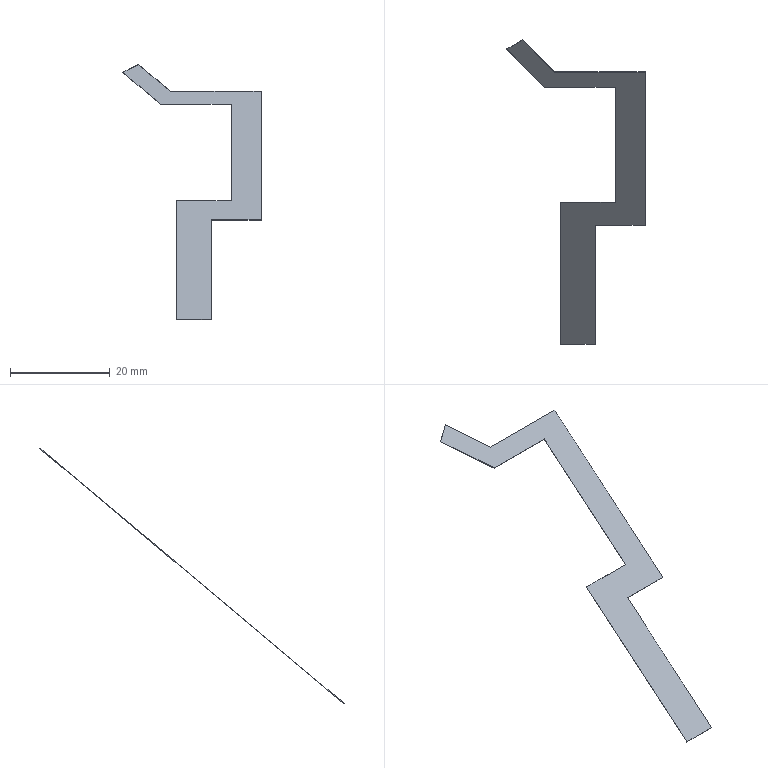Part | SolidWorks | features BaseBody 1 | 1 solid | 15 faces | box 27.714 x 60.861 x 51.086 mm | volume 46.633 mm3 | plane 15
STEP:
#1=CARTESIAN_POINT('',(-706.97,699.765,404.599));
#2=VERTEX_POINT('',#1);
#3=CARTESIAN_POINT('',(-710.165,697.921,403.051));
#4=VERTEX_POINT('',#3);
#5=CARTESIAN_POINT('',(-706.97,699.765,404.599));
#6=DIRECTION('',(-0.7986,-0.461,-0.3868));
#7=VECTOR('',#6,1000.);
#8=LINE('',#5,#7);
#9=EDGE_CURVE('',#2,#4,#8,.T.);
#10=ORIENTED_EDGE('',*,*,#9,.T.);
#11=CARTESIAN_POINT('',(-710.165,697.873,403.109));
#12=VERTEX_POINT('',#11);
#13=CARTESIAN_POINT('',(-710.165,697.873,403.109));
#14=DIRECTION('',(-0.000000993,0.6428,-0.766));
#15=VECTOR('',#14,1000.);
#16=LINE('',#13,#15);
#17=EDGE_CURVE('',#12,#4,#16,.T.);
#18=ORIENTED_EDGE('',*,*,#17,.F.);
#19=CARTESIAN_POINT('',(-706.97,699.717,404.656));
#20=VERTEX_POINT('',#19);
#21=CARTESIAN_POINT('',(-710.165,697.873,403.109));
#22=DIRECTION('',(0.7986,0.461,0.3868));
#23=VECTOR('',#22,1000.);
#24=LINE('',#21,#23);
#25=EDGE_CURVE('',#12,#20,#24,.T.);
#26=ORIENTED_EDGE('',*,*,#25,.T.);
#27=CARTESIAN_POINT('',(-706.97,699.765,404.599));
#28=DIRECTION('',(0.000000993,-0.6428,0.766));
#29=VECTOR('',#28,1000.);
#30=LINE('',#27,#29);
#31=EDGE_CURVE('',#2,#20,#30,.T.);
#32=ORIENTED_EDGE('',*,*,#31,.F.);
#33=EDGE_LOOP('',(#10,#18,#26,#32));
#34=FACE_OUTER_BOUND('',#33,.T.);
#35=CARTESIAN_POINT('',(-710.165,697.921,403.051));
#36=DIRECTION('',(0.6018,-0.6118,-0.5134));
#37=DIRECTION('',(0.7986,0.461,0.3868));
#38=AXIS2_PLACEMENT_3D('',#35,#36,#37);
#39=PLANE('',#38);
#40=ADVANCED_FACE('',(#34),#39,.F.);
#41=CARTESIAN_POINT('',(-700.651,693.342,399.208));
#42=VERTEX_POINT('',#41);
#43=CARTESIAN_POINT('',(-700.651,693.342,399.208));
#44=DIRECTION('',(-0.6018,0.6118,0.5134));
#45=VECTOR('',#44,1000.);
#46=LINE('',#43,#45);
#47=EDGE_CURVE('',#42,#2,#46,.T.);
#48=ORIENTED_EDGE('',*,*,#47,.T.);
#49=ORIENTED_EDGE('',*,*,#31,.T.);
#50=CARTESIAN_POINT('',(-700.651,693.293,399.266));
#51=VERTEX_POINT('',#50);
#52=CARTESIAN_POINT('',(-706.97,699.717,404.656));
#53=DIRECTION('',(0.6018,-0.6118,-0.5134));
#54=VECTOR('',#53,1000.);
#55=LINE('',#52,#54);
#56=EDGE_CURVE('',#20,#51,#55,.T.);
#57=ORIENTED_EDGE('',*,*,#56,.T.);
#58=CARTESIAN_POINT('',(-700.651,693.342,399.208));
#59=DIRECTION('',(0.000000993,-0.6428,0.766));
#60=VECTOR('',#59,1000.);
#61=LINE('',#58,#60);
#62=EDGE_CURVE('',#42,#51,#61,.T.);
#63=ORIENTED_EDGE('',*,*,#62,.F.);
#64=EDGE_LOOP('',(#48,#49,#57,#63));
#65=FACE_OUTER_BOUND('',#64,.T.);
#66=CARTESIAN_POINT('',(-706.97,699.765,404.599));
#67=DIRECTION('',(-0.7986,-0.461,-0.3868));
#68=DIRECTION('',(0.6018,-0.6118,-0.5134));
#69=AXIS2_PLACEMENT_3D('',#66,#67,#68);
#70=PLANE('',#69);
#71=ADVANCED_FACE('',(#65),#70,.F.);
#72=CARTESIAN_POINT('',(-688.451,693.342,399.208));
#73=VERTEX_POINT('',#72);
#74=CARTESIAN_POINT('',(-688.451,693.342,399.208));
#75=DIRECTION('',(-1.,-0.000001868,-0.000000272));
#76=VECTOR('',#75,1000.);
#77=LINE('',#74,#76);
#78=EDGE_CURVE('',#73,#42,#77,.T.);
#79=ORIENTED_EDGE('',*,*,#78,.T.);
#80=ORIENTED_EDGE('',*,*,#62,.T.);
#81=CARTESIAN_POINT('',(-688.451,693.293,399.266));
#82=VERTEX_POINT('',#81);
#83=CARTESIAN_POINT('',(-700.651,693.293,399.266));
#84=DIRECTION('',(1.,0.000001868,0.000000272));
#85=VECTOR('',#84,1000.);
#86=LINE('',#83,#85);
#87=EDGE_CURVE('',#51,#82,#86,.T.);
#88=ORIENTED_EDGE('',*,*,#87,.T.);
#89=CARTESIAN_POINT('',(-688.451,693.293,399.266));
#90=DIRECTION('',(-0.000000993,0.6428,-0.766));
#91=VECTOR('',#90,1000.);
#92=LINE('',#89,#91);
#93=EDGE_CURVE('',#82,#73,#92,.T.);
#94=ORIENTED_EDGE('',*,*,#93,.T.);
#95=EDGE_LOOP('',(#79,#80,#88,#94));
#96=FACE_OUTER_BOUND('',#95,.T.);
#97=CARTESIAN_POINT('',(-700.651,693.342,399.208));
#98=DIRECTION('',(0.000001866,-0.766,-0.6428));
#99=DIRECTION('',(1.,0.000002068,0.000000439));
#100=AXIS2_PLACEMENT_3D('',#97,#98,#99);
#101=PLANE('',#100);
#102=ADVANCED_FACE('',(#96),#101,.F.);
#103=CARTESIAN_POINT('',(-682.451,693.342,399.208));
#104=VERTEX_POINT('',#103);
#105=CARTESIAN_POINT('',(-682.451,693.342,399.208));
#106=DIRECTION('',(-1.,-0.000001661,-0.000000098));
#107=VECTOR('',#106,1000.);
#108=LINE('',#105,#107);
#109=EDGE_CURVE('',#104,#73,#108,.T.);
#110=ORIENTED_EDGE('',*,*,#109,.T.);
#111=ORIENTED_EDGE('',*,*,#93,.F.);
#112=CARTESIAN_POINT('',(-682.451,693.294,399.266));
#113=VERTEX_POINT('',#112);
#114=CARTESIAN_POINT('',(-688.451,693.293,399.266));
#115=DIRECTION('',(1.,0.000001661,0.000000098));
#116=VECTOR('',#115,1000.);
#117=LINE('',#114,#116);
#118=EDGE_CURVE('',#82,#113,#117,.T.);
#119=ORIENTED_EDGE('',*,*,#118,.T.);
#120=CARTESIAN_POINT('',(-682.451,693.294,399.266));
#121=DIRECTION('',(-0.000000993,0.6428,-0.766));
#122=VECTOR('',#121,1000.);
#123=LINE('',#120,#122);
#124=EDGE_CURVE('',#113,#104,#123,.T.);
#125=ORIENTED_EDGE('',*,*,#124,.T.);
#126=EDGE_LOOP('',(#110,#111,#119,#125));
#127=FACE_OUTER_BOUND('',#126,.T.);
#128=CARTESIAN_POINT('',(-688.451,693.342,399.208));
#129=DIRECTION('',(0.000001286,-0.766,-0.6428));
#130=DIRECTION('',(0.000000993,-0.6428,0.766));
#131=AXIS2_PLACEMENT_3D('',#128,#129,#130);
#132=PLANE('',#131);
#133=ADVANCED_FACE('',(#127),#132,.F.);
#134=CARTESIAN_POINT('',(-682.451,662.7,373.497));
#135=VERTEX_POINT('',#134);
#136=CARTESIAN_POINT('',(-682.451,662.7,373.497));
#137=DIRECTION('',(-0.000001286,0.766,0.6428));
#138=VECTOR('',#137,1000.);
#139=LINE('',#136,#138);
#140=EDGE_CURVE('',#135,#104,#139,.T.);
#141=ORIENTED_EDGE('',*,*,#140,.T.);
#142=ORIENTED_EDGE('',*,*,#124,.F.);
#143=CARTESIAN_POINT('',(-682.451,662.652,373.554));
#144=VERTEX_POINT('',#143);
#145=CARTESIAN_POINT('',(-682.451,693.294,399.266));
#146=DIRECTION('',(0.000001286,-0.766,-0.6428));
#147=VECTOR('',#146,1000.);
#148=LINE('',#145,#147);
#149=EDGE_CURVE('',#113,#144,#148,.T.);
#150=ORIENTED_EDGE('',*,*,#149,.T.);
#151=CARTESIAN_POINT('',(-682.451,662.652,373.554));
#152=DIRECTION('',(-0.000000993,0.6428,-0.766));
#153=VECTOR('',#152,1000.);
#154=LINE('',#151,#153);
#155=EDGE_CURVE('',#144,#135,#154,.T.);
#156=ORIENTED_EDGE('',*,*,#155,.T.);
#157=EDGE_LOOP('',(#141,#142,#150,#156));
#158=FACE_OUTER_BOUND('',#157,.T.);
#159=CARTESIAN_POINT('',(-682.451,693.342,399.208));
#160=DIRECTION('',(-1.,-0.000001623,-0.000000066));
#161=DIRECTION('',(0.000000993,-0.6428,0.766));
#162=AXIS2_PLACEMENT_3D('',#159,#160,#161);
#163=PLANE('',#162);
#164=ADVANCED_FACE('',(#158),#163,.F.);
#165=CARTESIAN_POINT('',(-692.451,662.7,373.497));
#166=VERTEX_POINT('',#165);
#167=CARTESIAN_POINT('',(-692.451,662.7,373.497));
#168=DIRECTION('',(1.,0.000001623,0.000000066));
#169=VECTOR('',#168,1000.);
#170=LINE('',#167,#169);
#171=EDGE_CURVE('',#166,#135,#170,.T.);
#172=ORIENTED_EDGE('',*,*,#171,.T.);
#173=ORIENTED_EDGE('',*,*,#155,.F.);
#174=CARTESIAN_POINT('',(-692.451,662.652,373.554));
#175=VERTEX_POINT('',#174);
#176=CARTESIAN_POINT('',(-682.451,662.652,373.554));
#177=DIRECTION('',(-1.,-0.000001623,-0.000000066));
#178=VECTOR('',#177,1000.);
#179=LINE('',#176,#178);
#180=EDGE_CURVE('',#144,#175,#179,.T.);
#181=ORIENTED_EDGE('',*,*,#180,.T.);
#182=CARTESIAN_POINT('',(-692.451,662.652,373.554));
#183=DIRECTION('',(-0.000000993,0.6428,-0.766));
#184=VECTOR('',#183,1000.);
#185=LINE('',#182,#184);
#186=EDGE_CURVE('',#175,#166,#185,.T.);
#187=ORIENTED_EDGE('',*,*,#186,.T.);
#188=EDGE_LOOP('',(#172,#173,#181,#187));
#189=FACE_OUTER_BOUND('',#188,.T.);
#190=CARTESIAN_POINT('',(-682.451,662.7,373.497));
#191=DIRECTION('',(-0.000001286,0.766,0.6428));
#192=DIRECTION('',(-0.000000993,0.6428,-0.766));
#193=AXIS2_PLACEMENT_3D('',#190,#191,#192);
#194=PLANE('',#193);
#195=ADVANCED_FACE('',(#189),#194,.F.);
#196=CARTESIAN_POINT('',(-692.451,638.953,353.571));
#197=VERTEX_POINT('',#196);
#198=CARTESIAN_POINT('',(-692.451,638.953,353.571));
#199=DIRECTION('',(-0.000001286,0.766,0.6428));
#200=VECTOR('',#199,1000.);
#201=LINE('',#198,#200);
#202=EDGE_CURVE('',#197,#166,#201,.T.);
#203=ORIENTED_EDGE('',*,*,#202,.T.);
#204=ORIENTED_EDGE('',*,*,#186,.F.);
#205=CARTESIAN_POINT('',(-692.451,638.904,353.628));
#206=VERTEX_POINT('',#205);
#207=CARTESIAN_POINT('',(-692.451,662.652,373.554));
#208=DIRECTION('',(0.000001286,-0.766,-0.6428));
#209=VECTOR('',#208,1000.);
#210=LINE('',#207,#209);
#211=EDGE_CURVE('',#175,#206,#210,.T.);
#212=ORIENTED_EDGE('',*,*,#211,.T.);
#213=CARTESIAN_POINT('',(-692.451,638.904,353.628));
#214=DIRECTION('',(-0.000000993,0.6428,-0.766));
#215=VECTOR('',#214,1000.);
#216=LINE('',#213,#215);
#217=EDGE_CURVE('',#206,#197,#216,.T.);
#218=ORIENTED_EDGE('',*,*,#217,.T.);
#219=EDGE_LOOP('',(#203,#204,#212,#218));
#220=FACE_OUTER_BOUND('',#219,.T.);
#221=CARTESIAN_POINT('',(-692.451,662.7,373.497));
#222=DIRECTION('',(-1.,-0.000001623,-0.000000066));
#223=DIRECTION('',(0.000000993,-0.6428,0.766));
#224=AXIS2_PLACEMENT_3D('',#221,#222,#223);
#225=PLANE('',#224);
#226=ADVANCED_FACE('',(#220),#225,.F.);
#227=CARTESIAN_POINT('',(-699.451,638.953,353.571));
#228=VERTEX_POINT('',#227);
#229=CARTESIAN_POINT('',(-699.451,638.953,353.571));
#230=DIRECTION('',(1.,0.000001623,0.000000066));
#231=VECTOR('',#230,1000.);
#232=LINE('',#229,#231);
#233=EDGE_CURVE('',#228,#197,#232,.T.);
#234=ORIENTED_EDGE('',*,*,#233,.T.);
#235=ORIENTED_EDGE('',*,*,#217,.F.);
#236=CARTESIAN_POINT('',(-699.451,638.904,353.628));
#237=VERTEX_POINT('',#236);
#238=CARTESIAN_POINT('',(-692.451,638.904,353.628));
#239=DIRECTION('',(-1.,-0.000001623,-0.000000066));
#240=VECTOR('',#239,1000.);
#241=LINE('',#238,#240);
#242=EDGE_CURVE('',#206,#237,#241,.T.);
#243=ORIENTED_EDGE('',*,*,#242,.T.);
#244=CARTESIAN_POINT('',(-699.451,638.904,353.628));
#245=DIRECTION('',(-0.000000993,0.6428,-0.766));
#246=VECTOR('',#245,1000.);
#247=LINE('',#244,#246);
#248=EDGE_CURVE('',#237,#228,#247,.T.);
#249=ORIENTED_EDGE('',*,*,#248,.T.);
#250=EDGE_LOOP('',(#234,#235,#243,#249));
#251=FACE_OUTER_BOUND('',#250,.T.);
#252=CARTESIAN_POINT('',(-692.451,638.953,353.571));
#253=DIRECTION('',(-0.000001286,0.766,0.6428));
#254=DIRECTION('',(-0.000000993,0.6428,-0.766));
#255=AXIS2_PLACEMENT_3D('',#252,#253,#254);
#256=PLANE('',#255);
#257=ADVANCED_FACE('',(#251),#256,.F.);
#258=CARTESIAN_POINT('',(-699.451,667.296,377.354));
#259=VERTEX_POINT('',#258);
#260=CARTESIAN_POINT('',(-699.451,667.296,377.354));
#261=DIRECTION('',(0.000001286,-0.766,-0.6428));
#262=VECTOR('',#261,1000.);
#263=LINE('',#260,#262);
#264=EDGE_CURVE('',#259,#228,#263,.T.);
#265=ORIENTED_EDGE('',*,*,#264,.T.);
#266=ORIENTED_EDGE('',*,*,#248,.F.);
#267=CARTESIAN_POINT('',(-699.451,667.248,377.411));
#268=VERTEX_POINT('',#267);
#269=CARTESIAN_POINT('',(-699.451,638.904,353.628));
#270=DIRECTION('',(-0.000001286,0.766,0.6428));
#271=VECTOR('',#270,1000.);
#272=LINE('',#269,#271);
#273=EDGE_CURVE('',#237,#268,#272,.T.);
#274=ORIENTED_EDGE('',*,*,#273,.T.);
#275=CARTESIAN_POINT('',(-699.451,667.248,377.411));
#276=DIRECTION('',(-0.000000993,0.6428,-0.766));
#277=VECTOR('',#276,1000.);
#278=LINE('',#275,#277);
#279=EDGE_CURVE('',#268,#259,#278,.T.);
#280=ORIENTED_EDGE('',*,*,#279,.T.);
#281=EDGE_LOOP('',(#265,#266,#274,#280));
#282=FACE_OUTER_BOUND('',#281,.T.);
#283=CARTESIAN_POINT('',(-699.451,644.315,358.07));
#284=DIRECTION('',(1.,0.000001623,0.000000066));
#285=DIRECTION('',(-0.000000993,0.6428,-0.766));
#286=AXIS2_PLACEMENT_3D('',#283,#284,#285);
#287=PLANE('',#286);
#288=ADVANCED_FACE('',(#282),#287,.F.);
#289=CARTESIAN_POINT('',(-688.451,667.296,377.354));
#290=VERTEX_POINT('',#289);
#291=CARTESIAN_POINT('',(-688.451,667.296,377.354));
#292=DIRECTION('',(-1.,-0.000001623,-0.000000066));
#293=VECTOR('',#292,1000.);
#294=LINE('',#291,#293);
#295=EDGE_CURVE('',#290,#259,#294,.T.);
#296=ORIENTED_EDGE('',*,*,#295,.T.);
#297=ORIENTED_EDGE('',*,*,#279,.F.);
#298=CARTESIAN_POINT('',(-688.451,667.248,377.411));
#299=VERTEX_POINT('',#298);
#300=CARTESIAN_POINT('',(-699.451,667.248,377.411));
#301=DIRECTION('',(1.,0.000001623,0.000000066));
#302=VECTOR('',#301,1000.);
#303=LINE('',#300,#302);
#304=EDGE_CURVE('',#268,#299,#303,.T.);
#305=ORIENTED_EDGE('',*,*,#304,.T.);
#306=CARTESIAN_POINT('',(-688.451,667.248,377.411));
#307=DIRECTION('',(-0.000000993,0.6428,-0.766));
#308=VECTOR('',#307,1000.);
#309=LINE('',#306,#308);
#310=EDGE_CURVE('',#299,#290,#309,.T.);
#311=ORIENTED_EDGE('',*,*,#310,.T.);
#312=EDGE_LOOP('',(#296,#297,#305,#311));
#313=FACE_OUTER_BOUND('',#312,.T.);
#314=CARTESIAN_POINT('',(-699.451,667.296,377.354));
#315=DIRECTION('',(0.000001286,-0.766,-0.6428));
#316=DIRECTION('',(0.000000993,-0.6428,0.766));
#317=AXIS2_PLACEMENT_3D('',#314,#315,#316);
#318=PLANE('',#317);
#319=ADVANCED_FACE('',(#313),#318,.F.);
#320=CARTESIAN_POINT('',(-688.451,690.278,396.637));
#321=VERTEX_POINT('',#320);
#322=CARTESIAN_POINT('',(-688.451,690.278,396.637));
#323=DIRECTION('',(0.000001286,-0.766,-0.6428));
#324=VECTOR('',#323,1000.);
#325=LINE('',#322,#324);
#326=EDGE_CURVE('',#321,#290,#325,.T.);
#327=ORIENTED_EDGE('',*,*,#326,.T.);
#328=ORIENTED_EDGE('',*,*,#310,.F.);
#329=CARTESIAN_POINT('',(-688.451,690.229,396.695));
#330=VERTEX_POINT('',#329);
#331=CARTESIAN_POINT('',(-688.451,667.248,377.411));
#332=DIRECTION('',(-0.000001286,0.766,0.6428));
#333=VECTOR('',#332,1000.);
#334=LINE('',#331,#333);
#335=EDGE_CURVE('',#299,#330,#334,.T.);
#336=ORIENTED_EDGE('',*,*,#335,.T.);
#337=CARTESIAN_POINT('',(-688.451,690.229,396.695));
#338=DIRECTION('',(-0.000000993,0.6428,-0.766));
#339=VECTOR('',#338,1000.);
#340=LINE('',#337,#339);
#341=EDGE_CURVE('',#330,#321,#340,.T.);
#342=ORIENTED_EDGE('',*,*,#341,.T.);
#343=EDGE_LOOP('',(#327,#328,#336,#342));
#344=FACE_OUTER_BOUND('',#343,.T.);
#345=CARTESIAN_POINT('',(-688.451,667.296,377.354));
#346=DIRECTION('',(1.,0.000001623,0.000000066));
#347=DIRECTION('',(-0.000000993,0.6428,-0.766));
#348=AXIS2_PLACEMENT_3D('',#345,#346,#347);
#349=PLANE('',#348);
#350=ADVANCED_FACE('',(#344),#349,.F.);
#351=CARTESIAN_POINT('',(-702.645,690.278,396.637));
#352=VERTEX_POINT('',#351);
#353=CARTESIAN_POINT('',(-702.645,690.278,396.637));
#354=DIRECTION('',(1.,0.000001824,0.000000234));
#355=VECTOR('',#354,1000.);
#356=LINE('',#353,#355);
#357=EDGE_CURVE('',#352,#321,#356,.T.);
#358=ORIENTED_EDGE('',*,*,#357,.T.);
#359=ORIENTED_EDGE('',*,*,#341,.F.);
#360=CARTESIAN_POINT('',(-702.645,690.229,396.695));
#361=VERTEX_POINT('',#360);
#362=CARTESIAN_POINT('',(-688.451,690.229,396.695));
#363=DIRECTION('',(-1.,-0.000001824,-0.000000234));
#364=VECTOR('',#363,1000.);
#365=LINE('',#362,#364);
#366=EDGE_CURVE('',#330,#361,#365,.T.);
#367=ORIENTED_EDGE('',*,*,#366,.T.);
#368=CARTESIAN_POINT('',(-702.645,690.229,396.695));
#369=DIRECTION('',(-0.000000993,0.6428,-0.766));
#370=VECTOR('',#369,1000.);
#371=LINE('',#368,#370);
#372=EDGE_CURVE('',#361,#352,#371,.T.);
#373=ORIENTED_EDGE('',*,*,#372,.T.);
#374=EDGE_LOOP('',(#358,#359,#367,#373));
#375=FACE_OUTER_BOUND('',#374,.T.);
#376=CARTESIAN_POINT('',(-688.451,690.278,396.637));
#377=DIRECTION('',(-0.000001866,0.766,0.6428));
#378=DIRECTION('',(-1.,-0.000002068,-0.000000439));
#379=AXIS2_PLACEMENT_3D('',#376,#377,#378);
#380=PLANE('',#379);
#381=ADVANCED_FACE('',(#375),#380,.F.);
#382=CARTESIAN_POINT('',(-710.165,697.921,403.051));
#383=DIRECTION('',(0.6018,-0.6118,-0.5134));
#384=VECTOR('',#383,1000.);
#385=LINE('',#382,#384);
#386=EDGE_CURVE('',#4,#352,#385,.T.);
#387=ORIENTED_EDGE('',*,*,#386,.T.);
#388=ORIENTED_EDGE('',*,*,#372,.F.);
#389=CARTESIAN_POINT('',(-702.645,690.229,396.695));
#390=DIRECTION('',(-0.6018,0.6118,0.5134));
#391=VECTOR('',#390,1000.);
#392=LINE('',#389,#391);
#393=EDGE_CURVE('',#361,#12,#392,.T.);
#394=ORIENTED_EDGE('',*,*,#393,.T.);
#395=ORIENTED_EDGE('',*,*,#17,.T.);
#396=EDGE_LOOP('',(#387,#388,#394,#395));
#397=FACE_OUTER_BOUND('',#396,.T.);
#398=CARTESIAN_POINT('',(-702.645,690.278,396.637));
#399=DIRECTION('',(0.7986,0.461,0.3868));
#400=DIRECTION('',(-0.6018,0.6118,0.5134));
#401=AXIS2_PLACEMENT_3D('',#398,#399,#400);
#402=PLANE('',#401);
#403=ADVANCED_FACE('',(#397),#402,.F.);
#404=ORIENTED_EDGE('',*,*,#366,.F.);
#405=ORIENTED_EDGE('',*,*,#335,.F.);
#406=ORIENTED_EDGE('',*,*,#304,.F.);
#407=ORIENTED_EDGE('',*,*,#273,.F.);
#408=ORIENTED_EDGE('',*,*,#242,.F.);
#409=ORIENTED_EDGE('',*,*,#211,.F.);
#410=ORIENTED_EDGE('',*,*,#180,.F.);
#411=ORIENTED_EDGE('',*,*,#149,.F.);
#412=ORIENTED_EDGE('',*,*,#118,.F.);
#413=ORIENTED_EDGE('',*,*,#87,.F.);
#414=ORIENTED_EDGE('',*,*,#56,.F.);
#415=ORIENTED_EDGE('',*,*,#25,.F.);
#416=ORIENTED_EDGE('',*,*,#393,.F.);
#417=EDGE_LOOP('',(#404,#405,#406,#407,#408,#409,#410,#411,#412,#413,#414,#415,#416));
#418=FACE_OUTER_BOUND('',#417,.T.);
#419=CARTESIAN_POINT('',(-733.13,689.217,395.846));
#420=DIRECTION('',(-0.000000993,0.6428,-0.766));
#421=DIRECTION('',(-1.,-0.000001623,-0.000000066));
#422=AXIS2_PLACEMENT_3D('',#419,#420,#421);
#423=PLANE('',#422);
#424=ADVANCED_FACE('',(#418),#423,.F.);
#425=ORIENTED_EDGE('',*,*,#78,.F.);
#426=ORIENTED_EDGE('',*,*,#109,.F.);
#427=ORIENTED_EDGE('',*,*,#140,.F.);
#428=ORIENTED_EDGE('',*,*,#171,.F.);
#429=ORIENTED_EDGE('',*,*,#202,.F.);
#430=ORIENTED_EDGE('',*,*,#233,.F.);
#431=ORIENTED_EDGE('',*,*,#264,.F.);
#432=ORIENTED_EDGE('',*,*,#295,.F.);
#433=ORIENTED_EDGE('',*,*,#326,.F.);
#434=ORIENTED_EDGE('',*,*,#357,.F.);
#435=ORIENTED_EDGE('',*,*,#386,.F.);
#436=ORIENTED_EDGE('',*,*,#9,.F.);
#437=ORIENTED_EDGE('',*,*,#47,.F.);
#438=EDGE_LOOP('',(#425,#426,#427,#428,#429,#430,#431,#432,#433,#434,#435,#436,#437));
#439=FACE_OUTER_BOUND('',#438,.T.);
#440=CARTESIAN_POINT('',(-733.13,689.266,395.788));
#441=DIRECTION('',(-0.000000993,0.6428,-0.766));
#442=DIRECTION('',(-1.,-0.000001623,-0.000000066));
#443=AXIS2_PLACEMENT_3D('',#440,#441,#442);
#444=PLANE('',#443);
#445=ADVANCED_FACE('',(#439),#444,.T.);
#446=CLOSED_SHELL('',(#40,#71,#102,#133,#164,#195,#226,#257,#288,#319,#350,#381,#403,#424,#445));
#447=MANIFOLD_SOLID_BREP('',#446);
#448=CARTESIAN_POINT('',(0.,0.,0.));
#449=DIRECTION('',(0.,0.,1.));
#450=DIRECTION('',(1.,0.,0.));
#451=AXIS2_PLACEMENT_3D('',#448,#449,#450);
#452=(LENGTH_UNIT()NAMED_UNIT(*)SI_UNIT(.MILLI.,.METRE.));
#453=UNCERTAINTY_MEASURE_WITH_UNIT(LENGTH_MEASURE(0.00001),#452,'','');
#454=(NAMED_UNIT(*)PLANE_ANGLE_UNIT()SI_UNIT($,.RADIAN.));
#455=(NAMED_UNIT(*)SI_UNIT($,.STERADIAN.)SOLID_ANGLE_UNIT());
#456=(GEOMETRIC_REPRESENTATION_CONTEXT(3)GLOBAL_UNCERTAINTY_ASSIGNED_CONTEXT((#453))GLOBAL_UNIT_ASSIGNED_CONTEXT((#452,#454,#455))REPRESENTATION_CONTEXT('',''));
#457=ADVANCED_BREP_SHAPE_REPRESENTATION('',(#447,#451),#456);